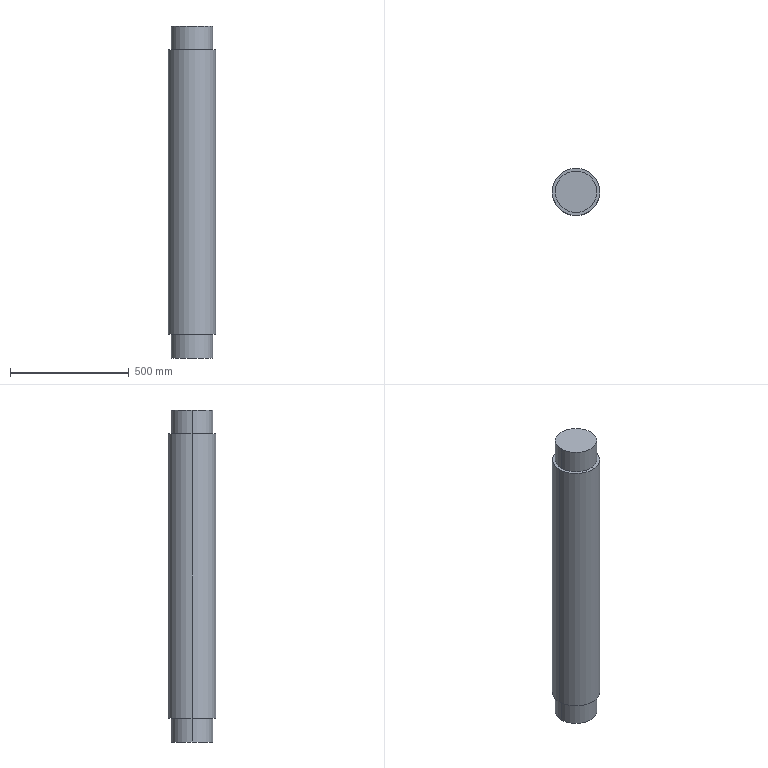Part | SolidWorks | features Extrusion 1, ICE 1 | 1 solid | 10 faces | box 200 x 200 x 1400 mm | volume 42509676 mm3 | cylinder 6 | plane 4 | commonest cylinder face diameters 175 x4 200 x2
STEP:
#1=CARTESIAN_POINT('',(87.5,0.,-600.));
#2=VERTEX_POINT('',#1);
#3=CARTESIAN_POINT('',(-87.5,0.,-600.));
#4=VERTEX_POINT('',#3);
#5=CARTESIAN_POINT('',(0.,0.,-600.));
#6=DIRECTION('',(0.,0.,1.));
#7=DIRECTION('',(1.,0.,0.));
#8=AXIS2_PLACEMENT_3D('',#5,#6,#7);
#9=CIRCLE('',#8,87.5);
#10=EDGE_CURVE('',#2,#4,#9,.T.);
#11=ORIENTED_EDGE('',*,*,#10,.F.);
#12=CARTESIAN_POINT('',(87.5,0.,-700.));
#13=VERTEX_POINT('',#12);
#14=CARTESIAN_POINT('',(87.5,0.,700.));
#15=DIRECTION('',(0.,0.,-1.));
#16=VECTOR('',#15,1000.);
#17=LINE('',#14,#16);
#18=EDGE_CURVE('',#2,#13,#17,.T.);
#19=ORIENTED_EDGE('',*,*,#18,.T.);
#20=CARTESIAN_POINT('',(-87.5,0.,-700.));
#21=VERTEX_POINT('',#20);
#22=CARTESIAN_POINT('',(0.,0.,-700.));
#23=DIRECTION('',(0.,0.,1.));
#24=DIRECTION('',(1.,0.,0.));
#25=AXIS2_PLACEMENT_3D('',#22,#23,#24);
#26=CIRCLE('',#25,87.5);
#27=EDGE_CURVE('',#13,#21,#26,.T.);
#28=ORIENTED_EDGE('',*,*,#27,.T.);
#29=CARTESIAN_POINT('',(-87.5,0.,700.));
#30=DIRECTION('',(0.,0.,-1.));
#31=VECTOR('',#30,1000.);
#32=LINE('',#29,#31);
#33=EDGE_CURVE('',#4,#21,#32,.T.);
#34=ORIENTED_EDGE('',*,*,#33,.F.);
#35=EDGE_LOOP('',(#11,#19,#28,#34));
#36=FACE_OUTER_BOUND('',#35,.T.);
#37=CARTESIAN_POINT('',(0.,0.,700.));
#38=DIRECTION('',(0.,0.,-1.));
#39=DIRECTION('',(-1.,0.,0.));
#40=AXIS2_PLACEMENT_3D('',#37,#38,#39);
#41=CYLINDRICAL_SURFACE('',#40,87.5);
#42=ADVANCED_FACE('',(#36),#41,.T.);
#43=CARTESIAN_POINT('',(100.,0.,600.));
#44=VERTEX_POINT('',#43);
#45=CARTESIAN_POINT('',(-100.,0.,600.));
#46=VERTEX_POINT('',#45);
#47=CARTESIAN_POINT('',(0.,0.,600.));
#48=DIRECTION('',(0.,0.,1.));
#49=DIRECTION('',(1.,0.,0.));
#50=AXIS2_PLACEMENT_3D('',#47,#48,#49);
#51=CIRCLE('',#50,100.);
#52=EDGE_CURVE('',#44,#46,#51,.T.);
#53=ORIENTED_EDGE('',*,*,#52,.F.);
#54=CARTESIAN_POINT('',(100.,0.,-600.));
#55=VERTEX_POINT('',#54);
#56=CARTESIAN_POINT('',(100.,0.,600.));
#57=DIRECTION('',(0.,0.,-1.));
#58=VECTOR('',#57,1000.);
#59=LINE('',#56,#58);
#60=EDGE_CURVE('',#44,#55,#59,.T.);
#61=ORIENTED_EDGE('',*,*,#60,.T.);
#62=CARTESIAN_POINT('',(-100.,0.,-600.));
#63=VERTEX_POINT('',#62);
#64=CARTESIAN_POINT('',(0.,0.,-600.));
#65=DIRECTION('',(0.,0.,1.));
#66=DIRECTION('',(1.,0.,0.));
#67=AXIS2_PLACEMENT_3D('',#64,#65,#66);
#68=CIRCLE('',#67,100.);
#69=EDGE_CURVE('',#55,#63,#68,.T.);
#70=ORIENTED_EDGE('',*,*,#69,.T.);
#71=CARTESIAN_POINT('',(-100.,0.,600.));
#72=DIRECTION('',(0.,0.,-1.));
#73=VECTOR('',#72,1000.);
#74=LINE('',#71,#73);
#75=EDGE_CURVE('',#46,#63,#74,.T.);
#76=ORIENTED_EDGE('',*,*,#75,.F.);
#77=EDGE_LOOP('',(#53,#61,#70,#76));
#78=FACE_OUTER_BOUND('',#77,.T.);
#79=CARTESIAN_POINT('',(0.,0.,600.));
#80=DIRECTION('',(0.,0.,-1.));
#81=DIRECTION('',(-1.,0.,0.));
#82=AXIS2_PLACEMENT_3D('',#79,#80,#81);
#83=CYLINDRICAL_SURFACE('',#82,100.);
#84=ADVANCED_FACE('',(#78),#83,.T.);
#85=CARTESIAN_POINT('',(87.5,0.,700.));
#86=VERTEX_POINT('',#85);
#87=CARTESIAN_POINT('',(-87.5,0.,700.));
#88=VERTEX_POINT('',#87);
#89=CARTESIAN_POINT('',(0.,0.,700.));
#90=DIRECTION('',(0.,0.,1.));
#91=DIRECTION('',(1.,0.,0.));
#92=AXIS2_PLACEMENT_3D('',#89,#90,#91);
#93=CIRCLE('',#92,87.5);
#94=EDGE_CURVE('',#86,#88,#93,.T.);
#95=ORIENTED_EDGE('',*,*,#94,.F.);
#96=CARTESIAN_POINT('',(87.5,0.,600.));
#97=VERTEX_POINT('',#96);
#98=CARTESIAN_POINT('',(87.5,0.,700.));
#99=DIRECTION('',(0.,0.,-1.));
#100=VECTOR('',#99,1000.);
#101=LINE('',#98,#100);
#102=EDGE_CURVE('',#86,#97,#101,.T.);
#103=ORIENTED_EDGE('',*,*,#102,.T.);
#104=CARTESIAN_POINT('',(-87.5,0.,600.));
#105=VERTEX_POINT('',#104);
#106=CARTESIAN_POINT('',(0.,0.,600.));
#107=DIRECTION('',(0.,0.,1.));
#108=DIRECTION('',(1.,0.,0.));
#109=AXIS2_PLACEMENT_3D('',#106,#107,#108);
#110=CIRCLE('',#109,87.5);
#111=EDGE_CURVE('',#97,#105,#110,.T.);
#112=ORIENTED_EDGE('',*,*,#111,.T.);
#113=CARTESIAN_POINT('',(-87.5,0.,700.));
#114=DIRECTION('',(0.,0.,-1.));
#115=VECTOR('',#114,1000.);
#116=LINE('',#113,#115);
#117=EDGE_CURVE('',#88,#105,#116,.T.);
#118=ORIENTED_EDGE('',*,*,#117,.F.);
#119=EDGE_LOOP('',(#95,#103,#112,#118));
#120=FACE_OUTER_BOUND('',#119,.T.);
#121=CARTESIAN_POINT('',(0.,0.,700.));
#122=DIRECTION('',(0.,0.,-1.));
#123=DIRECTION('',(-1.,0.,0.));
#124=AXIS2_PLACEMENT_3D('',#121,#122,#123);
#125=CYLINDRICAL_SURFACE('',#124,87.5);
#126=ADVANCED_FACE('',(#120),#125,.T.);
#127=ORIENTED_EDGE('',*,*,#102,.F.);
#128=CARTESIAN_POINT('',(0.,0.,700.));
#129=DIRECTION('',(0.,0.,1.));
#130=DIRECTION('',(1.,0.,0.));
#131=AXIS2_PLACEMENT_3D('',#128,#129,#130);
#132=CIRCLE('',#131,87.5);
#133=EDGE_CURVE('',#88,#86,#132,.T.);
#134=ORIENTED_EDGE('',*,*,#133,.F.);
#135=ORIENTED_EDGE('',*,*,#117,.T.);
#136=CARTESIAN_POINT('',(0.,0.,600.));
#137=DIRECTION('',(0.,0.,1.));
#138=DIRECTION('',(1.,0.,0.));
#139=AXIS2_PLACEMENT_3D('',#136,#137,#138);
#140=CIRCLE('',#139,87.5);
#141=EDGE_CURVE('',#105,#97,#140,.T.);
#142=ORIENTED_EDGE('',*,*,#141,.T.);
#143=EDGE_LOOP('',(#127,#134,#135,#142));
#144=FACE_OUTER_BOUND('',#143,.T.);
#145=CARTESIAN_POINT('',(0.,0.,700.));
#146=DIRECTION('',(0.,0.,-1.));
#147=DIRECTION('',(-1.,0.,0.));
#148=AXIS2_PLACEMENT_3D('',#145,#146,#147);
#149=CYLINDRICAL_SURFACE('',#148,87.5);
#150=ADVANCED_FACE('',(#144),#149,.T.);
#151=ORIENTED_EDGE('',*,*,#133,.T.);
#152=ORIENTED_EDGE('',*,*,#94,.T.);
#153=EDGE_LOOP('',(#151,#152));
#154=FACE_OUTER_BOUND('',#153,.T.);
#155=CARTESIAN_POINT('',(0.,0.,700.));
#156=DIRECTION('',(0.,0.,1.));
#157=DIRECTION('',(1.,0.,0.));
#158=AXIS2_PLACEMENT_3D('',#155,#156,#157);
#159=PLANE('',#158);
#160=ADVANCED_FACE('',(#154),#159,.T.);
#161=ORIENTED_EDGE('',*,*,#60,.F.);
#162=CARTESIAN_POINT('',(0.,0.,600.));
#163=DIRECTION('',(0.,0.,1.));
#164=DIRECTION('',(1.,0.,0.));
#165=AXIS2_PLACEMENT_3D('',#162,#163,#164);
#166=CIRCLE('',#165,100.);
#167=EDGE_CURVE('',#46,#44,#166,.T.);
#168=ORIENTED_EDGE('',*,*,#167,.F.);
#169=ORIENTED_EDGE('',*,*,#75,.T.);
#170=CARTESIAN_POINT('',(0.,0.,-600.));
#171=DIRECTION('',(0.,0.,1.));
#172=DIRECTION('',(1.,0.,0.));
#173=AXIS2_PLACEMENT_3D('',#170,#171,#172);
#174=CIRCLE('',#173,100.);
#175=EDGE_CURVE('',#63,#55,#174,.T.);
#176=ORIENTED_EDGE('',*,*,#175,.T.);
#177=EDGE_LOOP('',(#161,#168,#169,#176));
#178=FACE_OUTER_BOUND('',#177,.T.);
#179=CARTESIAN_POINT('',(0.,0.,600.));
#180=DIRECTION('',(0.,0.,-1.));
#181=DIRECTION('',(-1.,0.,0.));
#182=AXIS2_PLACEMENT_3D('',#179,#180,#181);
#183=CYLINDRICAL_SURFACE('',#182,100.);
#184=ADVANCED_FACE('',(#178),#183,.T.);
#185=ORIENTED_EDGE('',*,*,#141,.F.);
#186=ORIENTED_EDGE('',*,*,#111,.F.);
#187=EDGE_LOOP('',(#185,#186));
#188=FACE_BOUND('',#187,.T.);
#189=ORIENTED_EDGE('',*,*,#167,.T.);
#190=ORIENTED_EDGE('',*,*,#52,.T.);
#191=EDGE_LOOP('',(#189,#190));
#192=FACE_OUTER_BOUND('',#191,.T.);
#193=CARTESIAN_POINT('',(0.,0.,600.));
#194=DIRECTION('',(0.,0.,1.));
#195=DIRECTION('',(1.,0.,0.));
#196=AXIS2_PLACEMENT_3D('',#193,#194,#195);
#197=PLANE('',#196);
#198=ADVANCED_FACE('',(#188,#192),#197,.T.);
#199=CARTESIAN_POINT('',(0.,0.,-600.));
#200=DIRECTION('',(0.,0.,1.));
#201=DIRECTION('',(1.,0.,0.));
#202=AXIS2_PLACEMENT_3D('',#199,#200,#201);
#203=CIRCLE('',#202,87.5);
#204=EDGE_CURVE('',#4,#2,#203,.T.);
#205=ORIENTED_EDGE('',*,*,#204,.T.);
#206=ORIENTED_EDGE('',*,*,#10,.T.);
#207=EDGE_LOOP('',(#205,#206));
#208=FACE_BOUND('',#207,.T.);
#209=ORIENTED_EDGE('',*,*,#175,.F.);
#210=ORIENTED_EDGE('',*,*,#69,.F.);
#211=EDGE_LOOP('',(#209,#210));
#212=FACE_OUTER_BOUND('',#211,.T.);
#213=CARTESIAN_POINT('',(0.,0.,-600.));
#214=DIRECTION('',(0.,0.,1.));
#215=DIRECTION('',(1.,0.,0.));
#216=AXIS2_PLACEMENT_3D('',#213,#214,#215);
#217=PLANE('',#216);
#218=ADVANCED_FACE('',(#208,#212),#217,.F.);
#219=CARTESIAN_POINT('',(0.,0.,-700.));
#220=DIRECTION('',(0.,0.,1.));
#221=DIRECTION('',(1.,0.,0.));
#222=AXIS2_PLACEMENT_3D('',#219,#220,#221);
#223=CIRCLE('',#222,87.5);
#224=EDGE_CURVE('',#21,#13,#223,.T.);
#225=ORIENTED_EDGE('',*,*,#224,.F.);
#226=ORIENTED_EDGE('',*,*,#27,.F.);
#227=EDGE_LOOP('',(#225,#226));
#228=FACE_OUTER_BOUND('',#227,.T.);
#229=CARTESIAN_POINT('',(0.,0.,-700.));
#230=DIRECTION('',(0.,0.,1.));
#231=DIRECTION('',(1.,0.,0.));
#232=AXIS2_PLACEMENT_3D('',#229,#230,#231);
#233=PLANE('',#232);
#234=ADVANCED_FACE('',(#228),#233,.F.);
#235=ORIENTED_EDGE('',*,*,#18,.F.);
#236=ORIENTED_EDGE('',*,*,#204,.F.);
#237=ORIENTED_EDGE('',*,*,#33,.T.);
#238=ORIENTED_EDGE('',*,*,#224,.T.);
#239=EDGE_LOOP('',(#235,#236,#237,#238));
#240=FACE_OUTER_BOUND('',#239,.T.);
#241=CARTESIAN_POINT('',(0.,0.,700.));
#242=DIRECTION('',(0.,0.,-1.));
#243=DIRECTION('',(-1.,0.,0.));
#244=AXIS2_PLACEMENT_3D('',#241,#242,#243);
#245=CYLINDRICAL_SURFACE('',#244,87.5);
#246=ADVANCED_FACE('',(#240),#245,.T.);
#247=CLOSED_SHELL('',(#42,#84,#126,#150,#160,#184,#198,#218,#234,#246));
#248=MANIFOLD_SOLID_BREP('',#247);
#249=CARTESIAN_POINT('',(0.,0.,0.));
#250=DIRECTION('',(0.,0.,1.));
#251=DIRECTION('',(1.,0.,0.));
#252=AXIS2_PLACEMENT_3D('',#249,#250,#251);
#253=(LENGTH_UNIT()NAMED_UNIT(*)SI_UNIT(.MILLI.,.METRE.));
#254=UNCERTAINTY_MEASURE_WITH_UNIT(LENGTH_MEASURE(0.00001),#253,'','');
#255=(NAMED_UNIT(*)PLANE_ANGLE_UNIT()SI_UNIT($,.RADIAN.));
#256=(NAMED_UNIT(*)SI_UNIT($,.STERADIAN.)SOLID_ANGLE_UNIT());
#257=(GEOMETRIC_REPRESENTATION_CONTEXT(3)GLOBAL_UNCERTAINTY_ASSIGNED_CONTEXT((#254))GLOBAL_UNIT_ASSIGNED_CONTEXT((#253,#255,#256))REPRESENTATION_CONTEXT('',''));
#258=ADVANCED_BREP_SHAPE_REPRESENTATION('',(#248,#252),#257);